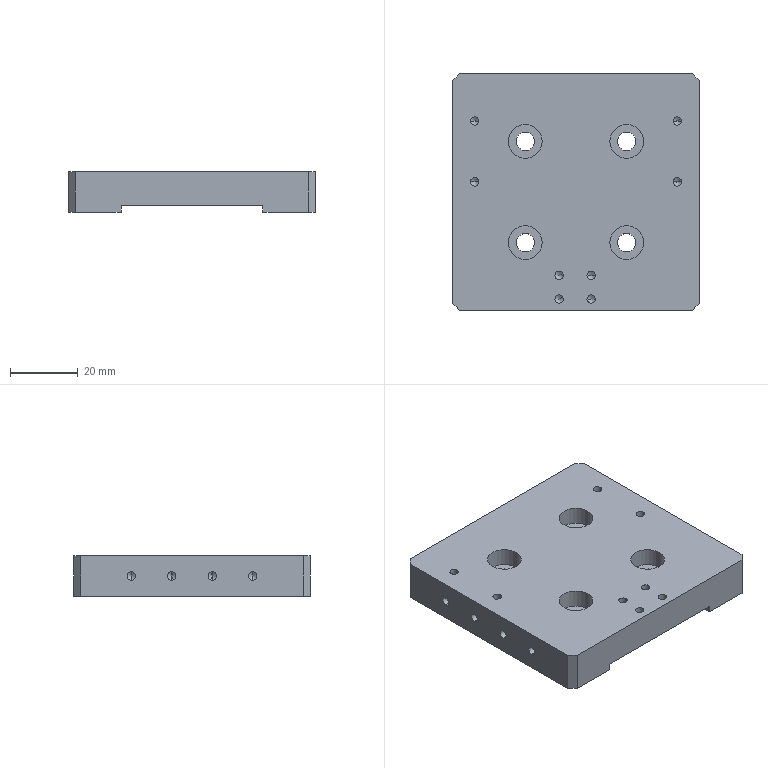Part | STEP file | 06-09KK60模组连接块 | 1 solid | 98 faces | box 73 x 70 x 12 mm | volume 52602 mm3 | cylinder 48 | cone 32 | plane 18 | commonest cylinder face diameters 2.5 x32 5.5 x8 10 x8